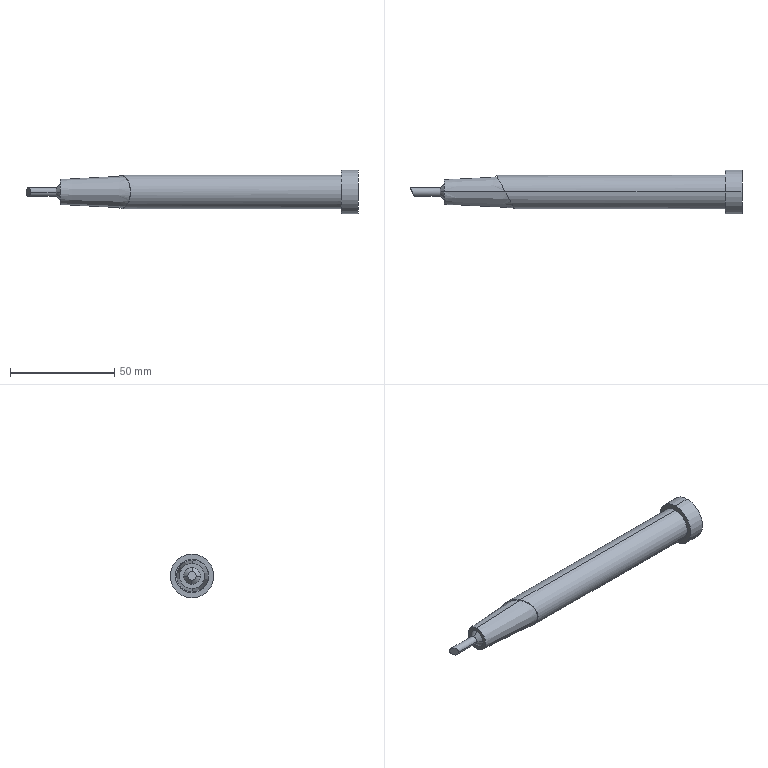Part | Creo | 1 solid | 17 faces | box 159.433 x 21 x 21 mm | volume 28475 mm3 | cylinder 6 | plane 5 | spline 4 | cone 2 | commonest cylinder face diameters 4.02 x2 16 x2 21 x2
STEP:
#1=CARTESIAN_POINT('',(0.,0.,0.));
#2=DIRECTION('',(0.,0.,1.));
#3=DIRECTION('',(1.,0.,0.));
#4=AXIS2_PLACEMENT_3D('',#1,#2,#3);
#5=CARTESIAN_POINT('',(286.206,-41.747,-34.219));
#6=VERTEX_POINT('',#5);
#7=CARTESIAN_POINT('',(290.526,-49.747,-42.219));
#8=VERTEX_POINT('',#7);
#9=CARTESIAN_POINT('',(286.206,-41.747,-34.718));
#10=CARTESIAN_POINT('',(286.256,-41.839,-35.701));
#11=CARTESIAN_POINT('',(286.478,-42.251,-37.148));
#12=CARTESIAN_POINT('',(286.853,-42.944,-38.521));
#13=CARTESIAN_POINT('',(287.359,-43.882,-39.731));
#14=CARTESIAN_POINT('',(287.99,-45.05,-40.76));
#15=CARTESIAN_POINT('',(288.754,-46.465,-41.578));
#16=CARTESIAN_POINT('',(289.619,-48.068,-42.1));
#17=CARTESIAN_POINT('',(290.218,-49.176,-42.219));
#18=CARTESIAN_POINT('',(290.526,-49.747,-42.219));
#19=B_SPLINE_CURVE_WITH_KNOTS('',3,(#5,#9,#10,#11,#12,#13,#14,#15,#16,#17,#18),.UNSPECIFIED.,.F.,.F.,(4,1,1,1,1,1,1,1,4),(0.,0.125,0.25,0.375,0.5,0.625,0.75,0.875,1.),.UNSPECIFIED.);
#20=EDGE_CURVE('',#6,#8,#19,.T.);
#21=ORIENTED_EDGE('',*,*,#20,.T.);
#22=CARTESIAN_POINT('',(396.101,-49.747,-42.219));
#23=VERTEX_POINT('',#22);
#24=CARTESIAN_POINT('',(290.526,-49.747,-42.219));
#25=DIRECTION('',(1.,0.000000001,-0.000000955));
#26=VECTOR('',#25,105.575);
#27=LINE('',#24,#26);
#28=EDGE_CURVE('',#8,#23,#27,.T.);
#29=ORIENTED_EDGE('',*,*,#28,.T.);
#30=CARTESIAN_POINT('',(396.101,-49.747,-26.219));
#31=VERTEX_POINT('',#30);
#32=CARTESIAN_POINT('',(396.101,-49.747,-34.219));
#33=DIRECTION('',(1.,0.,0.));
#34=DIRECTION('',(0.,0.,-1.));
#35=AXIS2_PLACEMENT_3D('',#32,#33,#34);
#36=CIRCLE('',#35,8.);
#37=EDGE_CURVE('',#23,#31,#36,.T.);
#38=ORIENTED_EDGE('',*,*,#37,.T.);
#39=CARTESIAN_POINT('',(290.526,-49.747,-26.219));
#40=VERTEX_POINT('',#39);
#41=CARTESIAN_POINT('',(290.526,-49.747,-26.219));
#42=DIRECTION('',(1.,0.00000261,0.000001073));
#43=VECTOR('',#42,105.574);
#44=LINE('',#41,#43);
#45=EDGE_CURVE('',#40,#31,#44,.T.);
#46=ORIENTED_EDGE('',*,*,#45,.F.);
#47=CARTESIAN_POINT('',(286.206,-41.747,-34.219));
#48=CARTESIAN_POINT('',(286.206,-41.747,-33.949));
#49=CARTESIAN_POINT('',(286.221,-41.774,-33.41));
#50=CARTESIAN_POINT('',(286.287,-41.897,-32.605));
#51=CARTESIAN_POINT('',(286.398,-42.103,-31.812));
#52=CARTESIAN_POINT('',(286.554,-42.391,-31.037));
#53=CARTESIAN_POINT('',(286.755,-42.764,-30.285));
#54=CARTESIAN_POINT('',(287.002,-43.22,-29.566));
#55=CARTESIAN_POINT('',(287.293,-43.76,-28.888));
#56=CARTESIAN_POINT('',(287.629,-44.381,-28.263));
#57=CARTESIAN_POINT('',(288.005,-45.079,-27.7));
#58=CARTESIAN_POINT('',(288.426,-45.858,-27.209));
#59=CARTESIAN_POINT('',(288.829,-46.603,-26.849));
#60=CARTESIAN_POINT('',(289.186,-47.266,-26.604));
#61=CARTESIAN_POINT('',(289.512,-47.869,-26.435));
#62=CARTESIAN_POINT('',(289.805,-48.41,-26.325));
#63=CARTESIAN_POINT('',(290.072,-48.905,-26.259));
#64=CARTESIAN_POINT('',(290.304,-49.335,-26.226));
#65=CARTESIAN_POINT('',(290.454,-49.613,-26.219));
#66=CARTESIAN_POINT('',(290.526,-49.747,-26.219));
#67=B_SPLINE_CURVE_WITH_KNOTS('',3,(#47,#48,#49,#50,#51,#52,#53,#54,#55,#56,#57,#58,#59,#60,#61,#62,#63,#64,#65,#66),.UNSPECIFIED.,.F.,.F.,(4,1,1,1,1,1,1,1,1,1,1,1,1,1,1,1,1,4),(0.,0.05882,0.1176,0.1765,0.2353,0.2941,0.3529,0.4118,0.4706,0.5294,0.5882,0.6471,0.7059,0.7647,0.8235,0.8824,0.9412,1.),.UNSPECIFIED.);
#68=EDGE_CURVE('',#6,#40,#67,.T.);
#69=ORIENTED_EDGE('',*,*,#68,.F.);
#70=EDGE_LOOP('',(#21,#29,#38,#46,#69));
#71=FACE_OUTER_BOUND('',#70,.F.);
#72=CARTESIAN_POINT('',(261.212,-49.747,-34.219));
#73=DIRECTION('',(1.,0.,0.));
#74=DIRECTION('',(0.,0.,-1.));
#75=AXIS2_PLACEMENT_3D('',#72,#73,#74);
#76=CYLINDRICAL_SURFACE('',#75,8.);
#77=ADVANCED_FACE('',(#71),#76,.T.);
#78=ORIENTED_EDGE('',*,*,#68,.T.);
#79=CARTESIAN_POINT('',(294.846,-57.747,-34.219));
#80=VERTEX_POINT('',#79);
#81=CARTESIAN_POINT('',(290.526,-49.747,-26.219));
#82=CARTESIAN_POINT('',(290.694,-50.058,-26.219));
#83=CARTESIAN_POINT('',(291.015,-50.651,-26.255));
#84=CARTESIAN_POINT('',(291.45,-51.458,-26.391));
#85=CARTESIAN_POINT('',(291.825,-52.152,-26.579));
#86=CARTESIAN_POINT('',(292.144,-52.743,-26.793));
#87=CARTESIAN_POINT('',(292.446,-53.301,-27.042));
#88=CARTESIAN_POINT('',(292.779,-53.918,-27.378));
#89=CARTESIAN_POINT('',(293.144,-54.594,-27.835));
#90=CARTESIAN_POINT('',(293.504,-55.261,-28.401));
#91=CARTESIAN_POINT('',(293.822,-55.849,-29.023));
#92=CARTESIAN_POINT('',(294.098,-56.361,-29.693));
#93=CARTESIAN_POINT('',(294.331,-56.793,-30.4));
#94=CARTESIAN_POINT('',(294.521,-57.144,-31.138));
#95=CARTESIAN_POINT('',(294.668,-57.416,-31.896));
#96=CARTESIAN_POINT('',(294.772,-57.61,-32.676));
#97=CARTESIAN_POINT('',(294.833,-57.721,-33.442));
#98=CARTESIAN_POINT('',(294.846,-57.747,-33.96));
#99=CARTESIAN_POINT('',(294.846,-57.747,-34.219));
#100=B_SPLINE_CURVE_WITH_KNOTS('',3,(#81,#82,#83,#84,#85,#86,#87,#88,#89,#90,#91,#92,#93,#94,#95,#96,#97,#98,#99),.UNSPECIFIED.,.F.,.F.,(4,1,1,1,1,1,1,1,1,1,1,1,1,1,1,1,4),(0.,0.0625,0.125,0.1875,0.25,0.3125,0.375,0.4375,0.5,0.5625,0.625,0.6875,0.75,0.8125,0.875,0.9375,1.),.UNSPECIFIED.);
#101=EDGE_CURVE('',#40,#80,#100,.T.);
#102=ORIENTED_EDGE('',*,*,#101,.T.);
#103=CARTESIAN_POINT('',(294.846,-57.747,-34.712));
#104=CARTESIAN_POINT('',(294.798,-57.657,-35.689));
#105=CARTESIAN_POINT('',(294.575,-57.243,-37.153));
#106=CARTESIAN_POINT('',(294.192,-56.535,-38.542));
#107=CARTESIAN_POINT('',(293.697,-55.618,-39.725));
#108=CARTESIAN_POINT('',(293.047,-54.415,-40.782));
#109=CARTESIAN_POINT('',(292.296,-53.023,-41.576));
#110=CARTESIAN_POINT('',(291.458,-51.472,-42.089));
#111=CARTESIAN_POINT('',(290.846,-50.339,-42.219));
#112=CARTESIAN_POINT('',(290.526,-49.747,-42.219));
#113=B_SPLINE_CURVE_WITH_KNOTS('',3,(#79,#103,#104,#105,#106,#107,#108,#109,#110,#111,#112),.UNSPECIFIED.,.F.,.F.,(4,1,1,1,1,1,1,1,4),(0.,0.125,0.25,0.375,0.5,0.625,0.75,0.875,1.),.UNSPECIFIED.);
#114=EDGE_CURVE('',#80,#8,#113,.T.);
#115=ORIENTED_EDGE('',*,*,#114,.T.);
#116=ORIENTED_EDGE('',*,*,#20,.F.);
#117=EDGE_LOOP('',(#78,#102,#115,#116));
#118=FACE_OUTER_BOUND('',#117,.F.);
#119=CARTESIAN_POINT('',(294.715,-57.503,-34.219));
#120=VERTEX_POINT('',#119);
#121=CARTESIAN_POINT('',(290.526,-49.747,-41.755));
#122=VERTEX_POINT('',#121);
#123=CARTESIAN_POINT('',(294.715,-57.503,-34.219));
#124=CARTESIAN_POINT('',(294.715,-57.503,-34.909));
#125=CARTESIAN_POINT('',(294.62,-57.327,-36.086));
#126=CARTESIAN_POINT('',(294.232,-56.608,-38.011));
#127=CARTESIAN_POINT('',(293.479,-55.215,-39.84));
#128=CARTESIAN_POINT('',(292.456,-53.32,-41.085));
#129=CARTESIAN_POINT('',(291.444,-51.446,-41.663));
#130=CARTESIAN_POINT('',(290.854,-50.354,-41.772));
#131=CARTESIAN_POINT('',(290.526,-49.747,-41.755));
#132=B_SPLINE_CURVE_WITH_KNOTS('',3,(#123,#124,#125,#126,#127,#128,#129,#130,#131),.UNSPECIFIED.,.F.,.F.,(4,1,1,1,1,1,4),(0.,0.125,0.25,0.5,0.75,0.875,1.),.UNSPECIFIED.);
#133=EDGE_CURVE('',#120,#122,#132,.T.);
#134=ORIENTED_EDGE('',*,*,#133,.F.);
#135=CARTESIAN_POINT('',(290.526,-49.747,-26.683));
#136=VERTEX_POINT('',#135);
#137=CARTESIAN_POINT('',(294.715,-57.503,-33.528));
#138=CARTESIAN_POINT('',(294.62,-57.327,-32.352));
#139=CARTESIAN_POINT('',(294.232,-56.608,-30.427));
#140=CARTESIAN_POINT('',(293.479,-55.215,-28.598));
#141=CARTESIAN_POINT('',(292.456,-53.32,-27.353));
#142=CARTESIAN_POINT('',(291.444,-51.446,-26.775));
#143=CARTESIAN_POINT('',(290.854,-50.354,-26.665));
#144=CARTESIAN_POINT('',(290.526,-49.747,-26.683));
#145=B_SPLINE_CURVE_WITH_KNOTS('',3,(#119,#137,#138,#139,#140,#141,#142,#143,#144),.UNSPECIFIED.,.F.,.F.,(4,1,1,1,1,1,4),(0.,0.125,0.25,0.5,0.75,0.875,1.),.UNSPECIFIED.);
#146=EDGE_CURVE('',#120,#136,#145,.T.);
#147=ORIENTED_EDGE('',*,*,#146,.T.);
#148=CARTESIAN_POINT('',(290.526,-49.747,-41.755));
#149=CARTESIAN_POINT('',(290.479,-49.66,-41.753));
#150=CARTESIAN_POINT('',(290.425,-49.559,-41.748));
#151=CARTESIAN_POINT('',(290.339,-49.399,-41.738));
#152=CARTESIAN_POINT('',(290.261,-49.256,-41.726));
#153=CARTESIAN_POINT('',(290.185,-49.114,-41.711));
#154=CARTESIAN_POINT('',(290.098,-48.953,-41.691));
#155=CARTESIAN_POINT('',(290.007,-48.785,-41.667));
#156=CARTESIAN_POINT('',(289.914,-48.612,-41.637));
#157=CARTESIAN_POINT('',(289.831,-48.46,-41.608));
#158=CARTESIAN_POINT('',(289.732,-48.276,-41.569));
#159=CARTESIAN_POINT('',(289.623,-48.073,-41.52));
#160=CARTESIAN_POINT('',(289.507,-47.859,-41.461));
#161=CARTESIAN_POINT('',(289.368,-47.602,-41.382));
#162=CARTESIAN_POINT('',(289.216,-47.321,-41.284));
#163=CARTESIAN_POINT('',(289.057,-47.026,-41.166));
#164=CARTESIAN_POINT('',(288.914,-46.762,-41.049));
#165=CARTESIAN_POINT('',(288.785,-46.522,-40.931));
#166=CARTESIAN_POINT('',(288.626,-46.228,-40.774));
#167=CARTESIAN_POINT('',(288.449,-45.9,-40.578));
#168=CARTESIAN_POINT('',(288.262,-45.554,-40.342));
#169=CARTESIAN_POINT('',(288.095,-45.244,-40.107));
#170=CARTESIAN_POINT('',(287.944,-44.965,-39.871));
#171=CARTESIAN_POINT('',(287.807,-44.71,-39.636));
#172=CARTESIAN_POINT('',(287.639,-44.4,-39.322));
#173=CARTESIAN_POINT('',(287.456,-44.061,-38.929));
#174=CARTESIAN_POINT('',(287.269,-43.714,-38.458));
#175=CARTESIAN_POINT('',(287.11,-43.42,-37.987));
#176=CARTESIAN_POINT('',(286.975,-43.171,-37.516));
#177=CARTESIAN_POINT('',(286.825,-42.892,-36.888));
#178=CARTESIAN_POINT('',(286.686,-42.636,-36.103));
#179=CARTESIAN_POINT('',(286.59,-42.457,-35.161));
#180=CARTESIAN_POINT('',(286.558,-42.398,-34.219));
#181=CARTESIAN_POINT('',(286.59,-42.457,-33.277));
#182=CARTESIAN_POINT('',(286.686,-42.636,-32.335));
#183=CARTESIAN_POINT('',(286.825,-42.892,-31.55));
#184=CARTESIAN_POINT('',(286.975,-43.171,-30.922));
#185=CARTESIAN_POINT('',(287.11,-43.42,-30.451));
#186=CARTESIAN_POINT('',(287.269,-43.714,-29.98));
#187=CARTESIAN_POINT('',(287.456,-44.061,-29.509));
#188=CARTESIAN_POINT('',(287.639,-44.4,-29.116));
#189=CARTESIAN_POINT('',(287.807,-44.71,-28.802));
#190=CARTESIAN_POINT('',(287.944,-44.965,-28.567));
#191=CARTESIAN_POINT('',(288.095,-45.244,-28.331));
#192=CARTESIAN_POINT('',(288.262,-45.554,-28.096));
#193=CARTESIAN_POINT('',(288.449,-45.9,-27.86));
#194=CARTESIAN_POINT('',(288.626,-46.228,-27.664));
#195=CARTESIAN_POINT('',(288.785,-46.522,-27.507));
#196=CARTESIAN_POINT('',(288.914,-46.762,-27.389));
#197=CARTESIAN_POINT('',(289.057,-47.026,-27.271));
#198=CARTESIAN_POINT('',(289.216,-47.321,-27.154));
#199=CARTESIAN_POINT('',(289.368,-47.602,-27.056));
#200=CARTESIAN_POINT('',(289.507,-47.859,-26.977));
#201=CARTESIAN_POINT('',(289.623,-48.073,-26.918));
#202=CARTESIAN_POINT('',(289.732,-48.276,-26.869));
#203=CARTESIAN_POINT('',(289.831,-48.46,-26.83));
#204=CARTESIAN_POINT('',(289.914,-48.612,-26.8));
#205=CARTESIAN_POINT('',(290.007,-48.785,-26.771));
#206=CARTESIAN_POINT('',(290.098,-48.953,-26.746));
#207=CARTESIAN_POINT('',(290.185,-49.114,-26.727));
#208=CARTESIAN_POINT('',(290.261,-49.256,-26.712));
#209=CARTESIAN_POINT('',(290.339,-49.399,-26.7));
#210=CARTESIAN_POINT('',(290.425,-49.559,-26.69));
#211=CARTESIAN_POINT('',(290.479,-49.66,-26.685));
#212=CARTESIAN_POINT('',(290.526,-49.747,-26.683));
#213=B_SPLINE_CURVE_WITH_KNOTS('',3,(#148,#149,#150,#151,#152,#153,#154,#155,#156,#157,#158,#159,#160,#161,#162,#163,#164,#165,#166,#167,#168,#169,#170,#171,#172,#173,#174,#175,#176,#177,#178,#179,#180,#181,#182,#183,#184,#185,#186,#187,#188,#189,#190,#191,#192,#193,#194,#195,#196,#197,#198,#199,#200,#201,#202,#203,#204,#205,#206,#207,#208,#209,#210,#211,#212),.UNSPECIFIED.,.F.,.F.,(4,1,1,1,1,1,1,1,1,1,1,1,1,1,1,1,1,1,1,1,1,1,1,1,1,1,1,1,1,1,1,1,1,1,1,1,1,1,1,1,1,1,1,1,1,1,1,1,1,1,1,1,1,1,1,1,1,1,1,1,1,1,4),(0.,0.0004883,0.0009766,0.001953,0.00293,0.003906,0.005859,0.007812,0.009766,0.01172,0.01562,0.01953,0.02344,0.03125,0.03906,0.04688,0.05469,0.0625,0.07812,0.09375,0.1094,0.125,0.1406,0.1562,0.1875,0.2188,0.25,0.2812,0.3125,0.375,0.4375,0.5,0.5625,0.625,0.6875,0.7188,0.75,0.7812,0.8125,0.8438,0.8594,0.875,0.8906,0.9062,0.9219,0.9375,0.9453,0.9531,0.9609,0.9688,0.9766,0.9805,0.9844,0.9883,0.9902,0.9922,0.9941,0.9961,0.9971,0.998,0.999,0.9995,1.),.UNSPECIFIED.);
#214=EDGE_CURVE('',#122,#136,#213,.T.);
#215=ORIENTED_EDGE('',*,*,#214,.F.);
#216=EDGE_LOOP('',(#134,#147,#215));
#217=FACE_BOUND('',#216,.F.);
#218=CARTESIAN_POINT('',(241.82,40.446,-130.777));
#219=DIRECTION('',(-0.8799,-0.4752,-0.000000028));
#220=DIRECTION('',(0.4752,-0.8799,0.));
#221=AXIS2_PLACEMENT_3D('',#218,#219,#220);
#222=PLANE('',#221);
#223=ADVANCED_FACE('',(#118,#217),#222,.T.);
#224=ORIENTED_EDGE('',*,*,#146,.F.);
#225=ORIENTED_EDGE('',*,*,#133,.T.);
#226=CARTESIAN_POINT('',(261.212,-49.747,-40.219));
#227=VERTEX_POINT('',#226);
#228=CARTESIAN_POINT('',(261.212,-49.747,-40.219));
#229=DIRECTION('',(0.9986,0.,-0.05234));
#230=VECTOR('',#229,29.354);
#231=LINE('',#228,#230);
#232=EDGE_CURVE('',#227,#122,#231,.T.);
#233=ORIENTED_EDGE('',*,*,#232,.F.);
#234=CARTESIAN_POINT('',(261.212,-49.747,-28.219));
#235=VERTEX_POINT('',#234);
#236=CARTESIAN_POINT('',(261.212,-49.747,-34.219));
#237=DIRECTION('',(-1.,0.,0.));
#238=DIRECTION('',(0.,0.,-1.));
#239=AXIS2_PLACEMENT_3D('',#236,#237,#238);
#240=CIRCLE('',#239,6.);
#241=EDGE_CURVE('',#227,#235,#240,.T.);
#242=ORIENTED_EDGE('',*,*,#241,.T.);
#243=CARTESIAN_POINT('',(261.212,-49.747,-28.219));
#244=DIRECTION('',(0.9986,0.,0.05234));
#245=VECTOR('',#244,29.354);
#246=LINE('',#243,#245);
#247=EDGE_CURVE('',#235,#136,#246,.T.);
#248=ORIENTED_EDGE('',*,*,#247,.T.);
#249=EDGE_LOOP('',(#224,#225,#233,#242,#248));
#250=FACE_OUTER_BOUND('',#249,.F.);
#251=CARTESIAN_POINT('',(277.963,-49.747,-34.219));
#252=DIRECTION('',(1.,0.,0.));
#253=DIRECTION('',(0.,0.,-1.));
#254=AXIS2_PLACEMENT_3D('',#251,#252,#253);
#255=CONICAL_SURFACE('',#254,6.878,3.);
#256=ADVANCED_FACE('',(#250),#255,.T.);
#257=ORIENTED_EDGE('',*,*,#214,.T.);
#258=ORIENTED_EDGE('',*,*,#247,.F.);
#259=CARTESIAN_POINT('',(261.212,-49.747,-34.219));
#260=DIRECTION('',(-1.,0.,0.));
#261=DIRECTION('',(0.,0.,1.));
#262=AXIS2_PLACEMENT_3D('',#259,#260,#261);
#263=CIRCLE('',#262,6.);
#264=EDGE_CURVE('',#235,#227,#263,.T.);
#265=ORIENTED_EDGE('',*,*,#264,.T.);
#266=ORIENTED_EDGE('',*,*,#232,.T.);
#267=EDGE_LOOP('',(#257,#258,#265,#266));
#268=FACE_OUTER_BOUND('',#267,.F.);
#269=CARTESIAN_POINT('',(275.869,-49.747,-34.219));
#270=DIRECTION('',(1.,0.,0.));
#271=DIRECTION('',(0.,0.,-1.));
#272=AXIS2_PLACEMENT_3D('',#269,#270,#271);
#273=CONICAL_SURFACE('',#272,6.768,3.);
#274=ADVANCED_FACE('',(#268),#273,.T.);
#275=ORIENTED_EDGE('',*,*,#241,.F.);
#276=ORIENTED_EDGE('',*,*,#264,.F.);
#277=EDGE_LOOP('',(#275,#276));
#278=FACE_OUTER_BOUND('',#277,.F.);
#279=CARTESIAN_POINT('',(261.212,-49.747,-30.199));
#280=VERTEX_POINT('',#279);
#281=CARTESIAN_POINT('',(261.212,-53.767,-34.219));
#282=VERTEX_POINT('',#281);
#283=CARTESIAN_POINT('',(261.212,-50.104,-30.199));
#284=CARTESIAN_POINT('',(261.212,-50.793,-30.295));
#285=CARTESIAN_POINT('',(261.212,-51.777,-30.702));
#286=CARTESIAN_POINT('',(261.212,-52.629,-31.351));
#287=CARTESIAN_POINT('',(261.212,-53.273,-32.203));
#288=CARTESIAN_POINT('',(261.212,-53.673,-33.183));
#289=CARTESIAN_POINT('',(261.212,-53.767,-33.866));
#290=CARTESIAN_POINT('',(261.212,-53.767,-34.219));
#291=B_SPLINE_CURVE_WITH_KNOTS('',3,(#279,#283,#284,#285,#286,#287,#288,#289,#290),.UNSPECIFIED.,.F.,.F.,(4,1,1,1,1,1,4),(0.,0.1667,0.3333,0.5,0.6667,0.8333,1.),.UNSPECIFIED.);
#292=EDGE_CURVE('',#280,#282,#291,.T.);
#293=ORIENTED_EDGE('',*,*,#292,.F.);
#294=CARTESIAN_POINT('',(261.212,-48.134,-30.537));
#295=VERTEX_POINT('',#294);
#296=CARTESIAN_POINT('',(261.212,-48.628,-30.32));
#297=CARTESIAN_POINT('',(261.212,-49.174,-30.199));
#298=CARTESIAN_POINT('',(261.212,-49.747,-30.199));
#299=B_SPLINE_CURVE_WITH_KNOTS('',3,(#294,#296,#297,#298),.UNSPECIFIED.,.F.,.F.,(4,4),(0.,1.),.UNSPECIFIED.);
#300=EDGE_CURVE('',#295,#280,#299,.T.);
#301=ORIENTED_EDGE('',*,*,#300,.F.);
#302=CARTESIAN_POINT('',(261.212,-46.588,-31.737));
#303=VERTEX_POINT('',#302);
#304=CARTESIAN_POINT('',(261.212,-46.994,-31.22));
#305=CARTESIAN_POINT('',(261.212,-47.525,-30.805));
#306=CARTESIAN_POINT('',(261.212,-48.134,-30.537));
#307=B_SPLINE_CURVE_WITH_KNOTS('',3,(#302,#304,#305,#306),.UNSPECIFIED.,.F.,.F.,(4,4),(0.,1.),.UNSPECIFIED.);
#308=EDGE_CURVE('',#303,#295,#307,.T.);
#309=ORIENTED_EDGE('',*,*,#308,.F.);
#310=CARTESIAN_POINT('',(261.212,-45.727,-34.219));
#311=VERTEX_POINT('',#310);
#312=CARTESIAN_POINT('',(261.212,-45.727,-33.917));
#313=CARTESIAN_POINT('',(261.212,-45.793,-33.33));
#314=CARTESIAN_POINT('',(261.212,-46.089,-32.476));
#315=CARTESIAN_POINT('',(261.212,-46.401,-31.974));
#316=CARTESIAN_POINT('',(261.212,-46.588,-31.737));
#317=B_SPLINE_CURVE_WITH_KNOTS('',3,(#310,#312,#313,#314,#315,#316),.UNSPECIFIED.,.F.,.F.,(4,1,1,4),(0.,0.3333,0.6667,1.),.UNSPECIFIED.);
#318=EDGE_CURVE('',#311,#303,#317,.T.);
#319=ORIENTED_EDGE('',*,*,#318,.F.);
#320=CARTESIAN_POINT('',(261.212,-49.747,-38.239));
#321=VERTEX_POINT('',#320);
#322=CARTESIAN_POINT('',(261.212,-49.39,-38.239));
#323=CARTESIAN_POINT('',(261.212,-48.701,-38.143));
#324=CARTESIAN_POINT('',(261.212,-47.717,-37.736));
#325=CARTESIAN_POINT('',(261.212,-46.864,-37.086));
#326=CARTESIAN_POINT('',(261.212,-46.221,-36.235));
#327=CARTESIAN_POINT('',(261.212,-45.82,-35.255));
#328=CARTESIAN_POINT('',(261.212,-45.727,-34.572));
#329=CARTESIAN_POINT('',(261.212,-45.727,-34.219));
#330=B_SPLINE_CURVE_WITH_KNOTS('',3,(#320,#322,#323,#324,#325,#326,#327,#328,#329),.UNSPECIFIED.,.F.,.F.,(4,1,1,1,1,1,4),(0.,0.1667,0.3333,0.5,0.6667,0.8333,1.),.UNSPECIFIED.);
#331=EDGE_CURVE('',#321,#311,#330,.T.);
#332=ORIENTED_EDGE('',*,*,#331,.F.);
#333=CARTESIAN_POINT('',(261.212,-53.767,-34.219));
#334=CARTESIAN_POINT('',(261.212,-53.767,-34.576));
#335=CARTESIAN_POINT('',(261.212,-53.671,-35.265));
#336=CARTESIAN_POINT('',(261.212,-53.264,-36.249));
#337=CARTESIAN_POINT('',(261.212,-52.614,-37.101));
#338=CARTESIAN_POINT('',(261.212,-51.763,-37.745));
#339=CARTESIAN_POINT('',(261.212,-50.783,-38.145));
#340=CARTESIAN_POINT('',(261.212,-50.1,-38.239));
#341=CARTESIAN_POINT('',(261.212,-49.747,-38.239));
#342=B_SPLINE_CURVE_WITH_KNOTS('',3,(#333,#334,#335,#336,#337,#338,#339,#340,#341),.UNSPECIFIED.,.F.,.F.,(4,1,1,1,1,1,4),(0.,0.1667,0.3333,0.5,0.6667,0.8333,1.),.UNSPECIFIED.);
#343=EDGE_CURVE('',#282,#321,#342,.T.);
#344=ORIENTED_EDGE('',*,*,#343,.F.);
#345=EDGE_LOOP('',(#293,#301,#309,#319,#332,#344));
#346=FACE_BOUND('',#345,.F.);
#347=CARTESIAN_POINT('',(261.212,-27.098,-27.127));
#348=DIRECTION('',(1.,-0.000000001,-0.00000112));
#349=DIRECTION('',(-0.00000112,0.,-1.));
#350=AXIS2_PLACEMENT_3D('',#347,#348,#349);
#351=PLANE('',#350);
#352=ADVANCED_FACE('',(#278,#346),#351,.F.);
#353=CARTESIAN_POINT('',(259.202,-49.747,-32.209));
#354=VERTEX_POINT('',#353);
#355=CARTESIAN_POINT('',(259.202,-51.757,-34.219));
#356=VERTEX_POINT('',#355);
#357=CARTESIAN_POINT('',(259.202,-49.747,-32.209));
#358=CARTESIAN_POINT('',(259.202,-49.959,-32.209));
#359=CARTESIAN_POINT('',(259.202,-50.381,-32.277));
#360=CARTESIAN_POINT('',(259.203,-50.949,-32.567));
#361=CARTESIAN_POINT('',(259.203,-51.399,-33.017));
#362=CARTESIAN_POINT('',(259.202,-51.689,-33.584));
#363=CARTESIAN_POINT('',(259.202,-51.757,-34.007));
#364=CARTESIAN_POINT('',(259.202,-51.757,-34.219));
#365=B_SPLINE_CURVE_WITH_KNOTS('',3,(#357,#358,#359,#360,#361,#362,#363,#364),.UNSPECIFIED.,.F.,.F.,(4,1,1,1,1,4),(0.,0.2,0.4,0.6,0.8,1.),.UNSPECIFIED.);
#366=EDGE_CURVE('',#354,#356,#365,.T.);
#367=ORIENTED_EDGE('',*,*,#366,.F.);
#368=CARTESIAN_POINT('',(261.212,-49.747,-30.199));
#369=DIRECTION('',(-0.7071,0.000000043,-0.7071));
#370=VECTOR('',#369,2.843);
#371=LINE('',#368,#370);
#372=EDGE_CURVE('',#280,#354,#371,.T.);
#373=ORIENTED_EDGE('',*,*,#372,.F.);
#374=ORIENTED_EDGE('',*,*,#292,.T.);
#375=CARTESIAN_POINT('',(259.202,-51.757,-34.219));
#376=DIRECTION('',(0.7071,-0.7071,-0.0000061));
#377=VECTOR('',#376,2.843);
#378=LINE('',#375,#377);
#379=EDGE_CURVE('',#356,#282,#378,.T.);
#380=ORIENTED_EDGE('',*,*,#379,.F.);
#381=EDGE_LOOP('',(#367,#373,#374,#380));
#382=FACE_OUTER_BOUND('',#381,.F.);
#383=CARTESIAN_POINT('',(259.064,-51.617,-34.305));
#384=CARTESIAN_POINT('',(259.826,-52.378,-34.34));
#385=CARTESIAN_POINT('',(260.588,-53.139,-34.375));
#386=CARTESIAN_POINT('',(261.35,-53.9,-34.41));
#387=CARTESIAN_POINT('',(259.064,-51.618,-34.276));
#388=CARTESIAN_POINT('',(259.826,-52.38,-34.3));
#389=CARTESIAN_POINT('',(260.588,-53.141,-34.323));
#390=CARTESIAN_POINT('',(261.35,-53.903,-34.346));
#391=CARTESIAN_POINT('',(259.064,-51.642,-33.21));
#392=CARTESIAN_POINT('',(259.826,-52.413,-32.8));
#393=CARTESIAN_POINT('',(260.588,-53.185,-32.389));
#394=CARTESIAN_POINT('',(261.35,-53.956,-31.979));
#395=CARTESIAN_POINT('',(259.064,-50.755,-32.323));
#396=CARTESIAN_POINT('',(259.826,-51.165,-31.552));
#397=CARTESIAN_POINT('',(260.588,-51.575,-30.78));
#398=CARTESIAN_POINT('',(261.35,-51.986,-30.009));
#399=CARTESIAN_POINT('',(259.064,-49.689,-32.347));
#400=CARTESIAN_POINT('',(259.826,-49.665,-31.586));
#401=CARTESIAN_POINT('',(260.588,-49.642,-30.824));
#402=CARTESIAN_POINT('',(261.35,-49.618,-30.063));
#403=CARTESIAN_POINT('',(259.064,-49.66,-32.349));
#404=CARTESIAN_POINT('',(259.826,-49.624,-31.588));
#405=CARTESIAN_POINT('',(260.588,-49.589,-30.827));
#406=CARTESIAN_POINT('',(261.35,-49.554,-30.066));
#407=B_SPLINE_SURFACE_WITH_KNOTS('',3,3,((#383,#384,#385,#386),(#387,#388,#389,#390),(#391,#392,#393,#394),(#395,#396,#397,#398),(#399,#400,#401,#402),(#403,#404,#405,#406)),.UNSPECIFIED.,.F.,.F.,.F.,(4,1,1,4),(4,4),(-0.02768,0.,1.,1.028),(-0.06858,1.068),.UNSPECIFIED.);
#408=ADVANCED_FACE('',(#382),#407,.F.);
#409=ORIENTED_EDGE('',*,*,#366,.T.);
#410=CARTESIAN_POINT('',(246.838,-51.757,-34.219));
#411=VERTEX_POINT('',#410);
#412=CARTESIAN_POINT('',(246.838,-51.757,-34.219));
#413=DIRECTION('',(1.,-0.000000968,-0.00000002));
#414=VECTOR('',#413,12.364);
#415=LINE('',#412,#414);
#416=EDGE_CURVE('',#411,#356,#415,.T.);
#417=ORIENTED_EDGE('',*,*,#416,.F.);
#418=CARTESIAN_POINT('',(246.647,-51.403,-33.08));
#419=VERTEX_POINT('',#418);
#420=CARTESIAN_POINT('',(246.838,-51.757,-34.219));
#421=CARTESIAN_POINT('',(246.838,-51.757,-34.085));
#422=CARTESIAN_POINT('',(246.825,-51.731,-33.821));
#423=CARTESIAN_POINT('',(246.76,-51.612,-33.439));
#424=CARTESIAN_POINT('',(246.69,-51.483,-33.196));
#425=B_SPLINE_CURVE_WITH_KNOTS('',3,(#420,#421,#422,#423,#424,#418),.UNSPECIFIED.,.F.,.F.,(4,1,1,4),(0.,0.3333,0.6667,1.),.UNSPECIFIED.);
#426=EDGE_CURVE('',#411,#419,#425,.T.);
#427=ORIENTED_EDGE('',*,*,#426,.T.);
#428=CARTESIAN_POINT('',(246.507,-51.143,-32.773));
#429=VERTEX_POINT('',#428);
#430=CARTESIAN_POINT('',(246.647,-51.403,-33.08));
#431=CARTESIAN_POINT('',(246.605,-51.325,-32.967));
#432=CARTESIAN_POINT('',(246.559,-51.239,-32.865));
#433=B_SPLINE_CURVE_WITH_KNOTS('',3,(#430,#431,#432,#428),.UNSPECIFIED.,.F.,.F.,(4,4),(0.,1.),.UNSPECIFIED.);
#434=EDGE_CURVE('',#419,#429,#433,.T.);
#435=ORIENTED_EDGE('',*,*,#434,.T.);
#436=CARTESIAN_POINT('',(244.667,-47.737,-34.219));
#437=VERTEX_POINT('',#436);
#438=CARTESIAN_POINT('',(246.507,-51.143,-32.773));
#439=CARTESIAN_POINT('',(246.429,-50.998,-32.633));
#440=CARTESIAN_POINT('',(246.257,-50.68,-32.406));
#441=CARTESIAN_POINT('',(245.944,-50.101,-32.209));
#442=CARTESIAN_POINT('',(245.61,-49.482,-32.195));
#443=CARTESIAN_POINT('',(245.286,-48.882,-32.371));
#444=CARTESIAN_POINT('',(245.013,-48.376,-32.71));
#445=CARTESIAN_POINT('',(244.812,-48.004,-33.166));
#446=CARTESIAN_POINT('',(244.693,-47.784,-33.684));
#447=CARTESIAN_POINT('',(244.667,-47.737,-34.037));
#448=CARTESIAN_POINT('',(244.667,-47.737,-34.219));
#449=B_SPLINE_CURVE_WITH_KNOTS('',3,(#438,#439,#440,#441,#442,#443,#444,#445,#446,#447,#448),.UNSPECIFIED.,.F.,.F.,(4,1,1,1,1,1,1,1,4),(0.,0.125,0.25,0.375,0.5,0.625,0.75,0.875,1.),.UNSPECIFIED.);
#450=EDGE_CURVE('',#429,#437,#449,.T.);
#451=ORIENTED_EDGE('',*,*,#450,.T.);
#452=CARTESIAN_POINT('',(259.202,-47.737,-34.219));
#453=VERTEX_POINT('',#452);
#454=CARTESIAN_POINT('',(244.667,-47.737,-34.219));
#455=DIRECTION('',(1.,-0.000001399,0.000000006));
#456=VECTOR('',#455,14.534);
#457=LINE('',#454,#456);
#458=EDGE_CURVE('',#437,#453,#457,.T.);
#459=ORIENTED_EDGE('',*,*,#458,.T.);
#460=CARTESIAN_POINT('',(259.202,-47.737,-34.219));
#461=CARTESIAN_POINT('',(259.202,-47.737,-34.007));
#462=CARTESIAN_POINT('',(259.202,-47.804,-33.584));
#463=CARTESIAN_POINT('',(259.203,-48.095,-33.017));
#464=CARTESIAN_POINT('',(259.203,-48.545,-32.567));
#465=CARTESIAN_POINT('',(259.202,-49.112,-32.277));
#466=CARTESIAN_POINT('',(259.202,-49.535,-32.209));
#467=CARTESIAN_POINT('',(259.202,-49.747,-32.209));
#468=B_SPLINE_CURVE_WITH_KNOTS('',3,(#460,#461,#462,#463,#464,#465,#466,#467),.UNSPECIFIED.,.F.,.F.,(4,1,1,1,1,4),(0.,0.2,0.4,0.6,0.8,1.),.UNSPECIFIED.);
#469=EDGE_CURVE('',#453,#354,#468,.T.);
#470=ORIENTED_EDGE('',*,*,#469,.T.);
#471=EDGE_LOOP('',(#409,#417,#427,#435,#451,#459,#470));
#472=FACE_OUTER_BOUND('',#471,.F.);
#473=CARTESIAN_POINT('',(245.672,-49.747,-34.219));
#474=DIRECTION('',(1.,0.,0.));
#475=DIRECTION('',(0.,1.,0.));
#476=AXIS2_PLACEMENT_3D('',#473,#474,#475);
#477=CYLINDRICAL_SURFACE('',#476,2.01);
#478=ADVANCED_FACE('',(#472),#477,.T.);
#479=CARTESIAN_POINT('',(259.202,-49.747,-36.229));
#480=VERTEX_POINT('',#479);
#481=CARTESIAN_POINT('',(259.202,-49.747,-36.229));
#482=CARTESIAN_POINT('',(259.202,-49.535,-36.229));
#483=CARTESIAN_POINT('',(259.202,-49.112,-36.161));
#484=CARTESIAN_POINT('',(259.203,-48.545,-35.871));
#485=CARTESIAN_POINT('',(259.203,-48.095,-35.421));
#486=CARTESIAN_POINT('',(259.202,-47.804,-34.853));
#487=CARTESIAN_POINT('',(259.202,-47.737,-34.431));
#488=CARTESIAN_POINT('',(259.202,-47.737,-34.219));
#489=B_SPLINE_CURVE_WITH_KNOTS('',3,(#481,#482,#483,#484,#485,#486,#487,#488),.UNSPECIFIED.,.F.,.F.,(4,1,1,1,1,4),(0.,0.2,0.4,0.6,0.8,1.),.UNSPECIFIED.);
#490=EDGE_CURVE('',#480,#453,#489,.T.);
#491=ORIENTED_EDGE('',*,*,#490,.T.);
#492=ORIENTED_EDGE('',*,*,#458,.F.);
#493=CARTESIAN_POINT('',(244.667,-47.737,-34.219));
#494=CARTESIAN_POINT('',(244.667,-47.737,-34.401));
#495=CARTESIAN_POINT('',(244.693,-47.785,-34.752));
#496=CARTESIAN_POINT('',(244.806,-47.993,-35.251));
#497=CARTESIAN_POINT('',(244.991,-48.336,-35.686));
#498=CARTESIAN_POINT('',(245.246,-48.808,-36.028));
#499=CARTESIAN_POINT('',(245.556,-49.381,-36.226));
#500=CARTESIAN_POINT('',(245.891,-50.003,-36.244));
#501=CARTESIAN_POINT('',(246.218,-50.608,-36.071));
#502=CARTESIAN_POINT('',(246.495,-51.122,-35.726));
#503=CARTESIAN_POINT('',(246.693,-51.488,-35.275));
#504=CARTESIAN_POINT('',(246.812,-51.708,-34.759));
#505=CARTESIAN_POINT('',(246.838,-51.757,-34.403));
#506=CARTESIAN_POINT('',(246.838,-51.757,-34.219));
#507=B_SPLINE_CURVE_WITH_KNOTS('',3,(#493,#494,#495,#496,#497,#498,#499,#500,#501,#502,#503,#504,#505,#506),.UNSPECIFIED.,.F.,.F.,(4,1,1,1,1,1,1,1,1,1,1,4),(0.,0.09091,0.1818,0.2727,0.3636,0.4545,0.5455,0.6364,0.7273,0.8182,0.9091,1.),.UNSPECIFIED.);
#508=EDGE_CURVE('',#437,#411,#507,.T.);
#509=ORIENTED_EDGE('',*,*,#508,.T.);
#510=ORIENTED_EDGE('',*,*,#416,.T.);
#511=CARTESIAN_POINT('',(259.202,-51.757,-34.219));
#512=CARTESIAN_POINT('',(259.202,-51.757,-34.431));
#513=CARTESIAN_POINT('',(259.202,-51.689,-34.853));
#514=CARTESIAN_POINT('',(259.203,-51.399,-35.421));
#515=CARTESIAN_POINT('',(259.203,-50.949,-35.871));
#516=CARTESIAN_POINT('',(259.202,-50.381,-36.161));
#517=CARTESIAN_POINT('',(259.202,-49.959,-36.229));
#518=CARTESIAN_POINT('',(259.202,-49.747,-36.229));
#519=B_SPLINE_CURVE_WITH_KNOTS('',3,(#511,#512,#513,#514,#515,#516,#517,#518),.UNSPECIFIED.,.F.,.F.,(4,1,1,1,1,4),(0.,0.2,0.4,0.6,0.8,1.),.UNSPECIFIED.);
#520=EDGE_CURVE('',#356,#480,#519,.T.);
#521=ORIENTED_EDGE('',*,*,#520,.T.);
#522=EDGE_LOOP('',(#491,#492,#509,#510,#521));
#523=FACE_OUTER_BOUND('',#522,.F.);
#524=CARTESIAN_POINT('',(245.672,-49.747,-34.219));
#525=DIRECTION('',(1.,0.,0.));
#526=DIRECTION('',(0.,1.,0.));
#527=AXIS2_PLACEMENT_3D('',#524,#525,#526);
#528=CYLINDRICAL_SURFACE('',#527,2.01);
#529=ADVANCED_FACE('',(#523),#528,.T.);
#530=ORIENTED_EDGE('',*,*,#490,.F.);
#531=CARTESIAN_POINT('',(259.202,-49.747,-36.229));
#532=DIRECTION('',(0.7071,0.00001227,-0.7071));
#533=VECTOR('',#532,2.843);
#534=LINE('',#531,#533);
#535=EDGE_CURVE('',#480,#321,#534,.T.);
#536=ORIENTED_EDGE('',*,*,#535,.T.);
#537=ORIENTED_EDGE('',*,*,#331,.T.);
#538=CARTESIAN_POINT('',(259.202,-47.737,-34.219));
#539=DIRECTION('',(0.7071,0.7071,-0.000001532));
#540=VECTOR('',#539,2.843);
#541=LINE('',#538,#540);
#542=EDGE_CURVE('',#453,#311,#541,.T.);
#543=ORIENTED_EDGE('',*,*,#542,.F.);
#544=EDGE_LOOP('',(#530,#536,#537,#543));
#545=FACE_OUTER_BOUND('',#544,.F.);
#546=CARTESIAN_POINT('',(259.064,-47.877,-34.133));
#547=CARTESIAN_POINT('',(259.826,-47.116,-34.098));
#548=CARTESIAN_POINT('',(260.588,-46.354,-34.063));
#549=CARTESIAN_POINT('',(261.35,-45.593,-34.028));
#550=CARTESIAN_POINT('',(259.064,-47.875,-34.162));
#551=CARTESIAN_POINT('',(259.826,-47.114,-34.138));
#552=CARTESIAN_POINT('',(260.588,-46.352,-34.115));
#553=CARTESIAN_POINT('',(261.35,-45.591,-34.092));
#554=CARTESIAN_POINT('',(259.064,-47.851,-35.228));
#555=CARTESIAN_POINT('',(259.826,-47.08,-35.638));
#556=CARTESIAN_POINT('',(260.588,-46.309,-36.048));
#557=CARTESIAN_POINT('',(261.35,-45.537,-36.459));
#558=CARTESIAN_POINT('',(259.064,-48.739,-36.115));
#559=CARTESIAN_POINT('',(259.826,-48.328,-36.886));
#560=CARTESIAN_POINT('',(260.588,-47.918,-37.657));
#561=CARTESIAN_POINT('',(261.35,-47.508,-38.429));
#562=CARTESIAN_POINT('',(259.064,-49.805,-36.09));
#563=CARTESIAN_POINT('',(259.826,-49.828,-36.852));
#564=CARTESIAN_POINT('',(260.588,-49.852,-37.614));
#565=CARTESIAN_POINT('',(261.35,-49.875,-38.375));
#566=CARTESIAN_POINT('',(259.064,-49.834,-36.089));
#567=CARTESIAN_POINT('',(259.826,-49.869,-36.85));
#568=CARTESIAN_POINT('',(260.588,-49.905,-37.611));
#569=CARTESIAN_POINT('',(261.35,-49.94,-38.372));
#570=B_SPLINE_SURFACE_WITH_KNOTS('',3,3,((#546,#547,#548,#549),(#550,#551,#552,#553),(#554,#555,#556,#557),(#558,#559,#560,#561),(#562,#563,#564,#565),(#566,#567,#568,#569)),.UNSPECIFIED.,.F.,.F.,.F.,(4,1,1,4),(4,4),(-0.02768,0.,1.,1.028),(-0.06858,1.068),.UNSPECIFIED.);
#571=ADVANCED_FACE('',(#545),#570,.F.);
#572=ORIENTED_EDGE('',*,*,#520,.F.);
#573=ORIENTED_EDGE('',*,*,#379,.T.);
#574=ORIENTED_EDGE('',*,*,#343,.T.);
#575=ORIENTED_EDGE('',*,*,#535,.F.);
#576=EDGE_LOOP('',(#572,#573,#574,#575));
#577=FACE_OUTER_BOUND('',#576,.F.);
#578=CARTESIAN_POINT('',(259.064,-49.661,-36.089));
#579=CARTESIAN_POINT('',(259.826,-49.626,-36.85));
#580=CARTESIAN_POINT('',(260.588,-49.591,-37.611));
#581=CARTESIAN_POINT('',(261.35,-49.556,-38.372));
#582=CARTESIAN_POINT('',(259.064,-49.689,-36.09));
#583=CARTESIAN_POINT('',(259.826,-49.666,-36.852));
#584=CARTESIAN_POINT('',(260.588,-49.643,-37.614));
#585=CARTESIAN_POINT('',(261.35,-49.62,-38.375));
#586=CARTESIAN_POINT('',(259.064,-50.755,-36.114));
#587=CARTESIAN_POINT('',(259.826,-51.166,-36.886));
#588=CARTESIAN_POINT('',(260.588,-51.576,-37.657));
#589=CARTESIAN_POINT('',(261.35,-51.987,-38.428));
#590=CARTESIAN_POINT('',(259.064,-51.642,-35.227));
#591=CARTESIAN_POINT('',(259.826,-52.414,-35.637));
#592=CARTESIAN_POINT('',(260.588,-53.185,-36.048));
#593=CARTESIAN_POINT('',(261.35,-53.957,-36.458));
#594=CARTESIAN_POINT('',(259.064,-51.618,-34.161));
#595=CARTESIAN_POINT('',(259.826,-52.38,-34.138));
#596=CARTESIAN_POINT('',(260.588,-53.141,-34.114));
#597=CARTESIAN_POINT('',(261.35,-53.903,-34.09));
#598=CARTESIAN_POINT('',(259.064,-51.617,-34.132));
#599=CARTESIAN_POINT('',(259.826,-52.378,-34.097));
#600=CARTESIAN_POINT('',(260.588,-53.139,-34.061));
#601=CARTESIAN_POINT('',(261.35,-53.9,-34.026));
#602=B_SPLINE_SURFACE_WITH_KNOTS('',3,3,((#578,#579,#580,#581),(#582,#583,#584,#585),(#586,#587,#588,#589),(#590,#591,#592,#593),(#594,#595,#596,#597),(#598,#599,#600,#601)),.UNSPECIFIED.,.F.,.F.,.F.,(4,1,1,4),(4,4),(-0.02768,0.,1.,1.028),(-0.06858,1.068),.UNSPECIFIED.);
#603=ADVANCED_FACE('',(#577),#602,.F.);
#604=ORIENTED_EDGE('',*,*,#469,.F.);
#605=ORIENTED_EDGE('',*,*,#542,.T.);
#606=ORIENTED_EDGE('',*,*,#318,.T.);
#607=ORIENTED_EDGE('',*,*,#308,.T.);
#608=ORIENTED_EDGE('',*,*,#300,.T.);
#609=ORIENTED_EDGE('',*,*,#372,.T.);
#610=EDGE_LOOP('',(#604,#605,#606,#607,#608,#609));
#611=FACE_OUTER_BOUND('',#610,.F.);
#612=CARTESIAN_POINT('',(259.064,-49.833,-32.349));
#613=CARTESIAN_POINT('',(259.826,-49.868,-31.588));
#614=CARTESIAN_POINT('',(260.588,-49.903,-30.827));
#615=CARTESIAN_POINT('',(261.35,-49.938,-30.065));
#616=CARTESIAN_POINT('',(259.064,-49.804,-32.347));
#617=CARTESIAN_POINT('',(259.826,-49.827,-31.586));
#618=CARTESIAN_POINT('',(260.588,-49.851,-30.824));
#619=CARTESIAN_POINT('',(261.35,-49.874,-30.063));
#620=CARTESIAN_POINT('',(259.064,-48.738,-32.324));
#621=CARTESIAN_POINT('',(259.826,-48.328,-31.552));
#622=CARTESIAN_POINT('',(260.588,-47.917,-30.781));
#623=CARTESIAN_POINT('',(261.35,-47.507,-30.01));
#624=CARTESIAN_POINT('',(259.064,-47.851,-33.211));
#625=CARTESIAN_POINT('',(259.826,-47.08,-32.801));
#626=CARTESIAN_POINT('',(260.588,-46.308,-32.39));
#627=CARTESIAN_POINT('',(261.35,-45.537,-31.98));
#628=CARTESIAN_POINT('',(259.064,-47.875,-34.277));
#629=CARTESIAN_POINT('',(259.826,-47.114,-34.3));
#630=CARTESIAN_POINT('',(260.588,-46.352,-34.324));
#631=CARTESIAN_POINT('',(261.35,-45.59,-34.347));
#632=CARTESIAN_POINT('',(259.064,-47.877,-34.306));
#633=CARTESIAN_POINT('',(259.826,-47.116,-34.341));
#634=CARTESIAN_POINT('',(260.588,-46.354,-34.377));
#635=CARTESIAN_POINT('',(261.35,-45.593,-34.412));
#636=B_SPLINE_SURFACE_WITH_KNOTS('',3,3,((#612,#613,#614,#615),(#616,#617,#618,#619),(#620,#621,#622,#623),(#624,#625,#626,#627),(#628,#629,#630,#631),(#632,#633,#634,#635)),.UNSPECIFIED.,.F.,.F.,.F.,(4,1,1,4),(4,4),(-0.02768,0.,1.,1.028),(-0.06858,1.069),.UNSPECIFIED.);
#637=ADVANCED_FACE('',(#611),#636,.F.);
#638=ORIENTED_EDGE('',*,*,#426,.F.);
#639=ORIENTED_EDGE('',*,*,#508,.F.);
#640=ORIENTED_EDGE('',*,*,#450,.F.);
#641=ORIENTED_EDGE('',*,*,#434,.F.);
#642=EDGE_LOOP('',(#638,#639,#640,#641));
#643=FACE_OUTER_BOUND('',#642,.F.);
#644=CARTESIAN_POINT('',(239.719,-38.574,-41.231));
#645=DIRECTION('',(-0.8799,-0.4752,-0.000000028));
#646=DIRECTION('',(0.4752,-0.8799,0.));
#647=AXIS2_PLACEMENT_3D('',#644,#645,#646);
#648=PLANE('',#647);
#649=ADVANCED_FACE('',(#643),#648,.T.);
#650=ORIENTED_EDGE('',*,*,#114,.F.);
#651=ORIENTED_EDGE('',*,*,#101,.F.);
#652=ORIENTED_EDGE('',*,*,#45,.T.);
#653=CARTESIAN_POINT('',(396.101,-49.747,-34.219));
#654=DIRECTION('',(1.,0.,0.));
#655=DIRECTION('',(0.,0.,1.));
#656=AXIS2_PLACEMENT_3D('',#653,#654,#655);
#657=CIRCLE('',#656,8.);
#658=EDGE_CURVE('',#31,#23,#657,.T.);
#659=ORIENTED_EDGE('',*,*,#658,.T.);
#660=ORIENTED_EDGE('',*,*,#28,.F.);
#661=EDGE_LOOP('',(#650,#651,#652,#659,#660));
#662=FACE_OUTER_BOUND('',#661,.F.);
#663=CARTESIAN_POINT('',(261.212,-49.747,-34.219));
#664=DIRECTION('',(1.,0.,0.));
#665=DIRECTION('',(0.,0.,-1.));
#666=AXIS2_PLACEMENT_3D('',#663,#664,#665);
#667=CYLINDRICAL_SURFACE('',#666,8.);
#668=ADVANCED_FACE('',(#662),#667,.T.);
#669=CARTESIAN_POINT('',(396.101,-49.747,-44.719));
#670=VERTEX_POINT('',#669);
#671=CARTESIAN_POINT('',(396.101,-49.747,-23.719));
#672=VERTEX_POINT('',#671);
#673=CARTESIAN_POINT('',(396.101,-49.747,-34.219));
#674=DIRECTION('',(-1.,0.,0.));
#675=DIRECTION('',(0.,0.,-1.));
#676=AXIS2_PLACEMENT_3D('',#673,#674,#675);
#677=CIRCLE('',#676,10.5);
#678=EDGE_CURVE('',#670,#672,#677,.T.);
#679=ORIENTED_EDGE('',*,*,#678,.F.);
#680=CARTESIAN_POINT('',(396.101,-49.747,-34.219));
#681=DIRECTION('',(-1.,0.,0.));
#682=DIRECTION('',(0.,0.,1.));
#683=AXIS2_PLACEMENT_3D('',#680,#681,#682);
#684=CIRCLE('',#683,10.5);
#685=EDGE_CURVE('',#672,#670,#684,.T.);
#686=ORIENTED_EDGE('',*,*,#685,.F.);
#687=EDGE_LOOP('',(#679,#686));
#688=FACE_OUTER_BOUND('',#687,.F.);
#689=ORIENTED_EDGE('',*,*,#37,.F.);
#690=ORIENTED_EDGE('',*,*,#658,.F.);
#691=EDGE_LOOP('',(#689,#690));
#692=FACE_BOUND('',#691,.F.);
#693=CARTESIAN_POINT('',(396.101,-49.747,-34.219));
#694=DIRECTION('',(1.,0.,0.));
#695=DIRECTION('',(0.,0.,-1.));
#696=AXIS2_PLACEMENT_3D('',#693,#694,#695);
#697=PLANE('',#696);
#698=ADVANCED_FACE('',(#688,#692),#697,.F.);
#699=ORIENTED_EDGE('',*,*,#678,.T.);
#700=CARTESIAN_POINT('',(404.101,-49.747,-23.719));
#701=VERTEX_POINT('',#700);
#702=CARTESIAN_POINT('',(396.101,-49.747,-23.719));
#703=DIRECTION('',(1.,0.,0.));
#704=VECTOR('',#703,8.);
#705=LINE('',#702,#704);
#706=EDGE_CURVE('',#672,#701,#705,.T.);
#707=ORIENTED_EDGE('',*,*,#706,.T.);
#708=CARTESIAN_POINT('',(404.101,-49.747,-44.719));
#709=VERTEX_POINT('',#708);
#710=CARTESIAN_POINT('',(404.101,-49.747,-34.219));
#711=DIRECTION('',(1.,0.,0.));
#712=DIRECTION('',(0.,0.,1.));
#713=AXIS2_PLACEMENT_3D('',#710,#711,#712);
#714=CIRCLE('',#713,10.5);
#715=EDGE_CURVE('',#701,#709,#714,.T.);
#716=ORIENTED_EDGE('',*,*,#715,.T.);
#717=CARTESIAN_POINT('',(396.101,-49.747,-44.719));
#718=DIRECTION('',(1.,0.,0.));
#719=VECTOR('',#718,8.);
#720=LINE('',#717,#719);
#721=EDGE_CURVE('',#670,#709,#720,.T.);
#722=ORIENTED_EDGE('',*,*,#721,.F.);
#723=EDGE_LOOP('',(#699,#707,#716,#722));
#724=FACE_OUTER_BOUND('',#723,.F.);
#725=CARTESIAN_POINT('',(421.101,-49.747,-34.219));
#726=DIRECTION('',(1.,0.,0.));
#727=DIRECTION('',(0.,0.,-1.));
#728=AXIS2_PLACEMENT_3D('',#725,#726,#727);
#729=CYLINDRICAL_SURFACE('',#728,10.5);
#730=ADVANCED_FACE('',(#724),#729,.T.);
#731=ORIENTED_EDGE('',*,*,#685,.T.);
#732=ORIENTED_EDGE('',*,*,#721,.T.);
#733=CARTESIAN_POINT('',(404.101,-49.747,-34.219));
#734=DIRECTION('',(1.,0.,0.));
#735=DIRECTION('',(0.,0.,-1.));
#736=AXIS2_PLACEMENT_3D('',#733,#734,#735);
#737=CIRCLE('',#736,10.5);
#738=EDGE_CURVE('',#709,#701,#737,.T.);
#739=ORIENTED_EDGE('',*,*,#738,.T.);
#740=ORIENTED_EDGE('',*,*,#706,.F.);
#741=EDGE_LOOP('',(#731,#732,#739,#740));
#742=FACE_OUTER_BOUND('',#741,.F.);
#743=CARTESIAN_POINT('',(421.101,-49.747,-34.219));
#744=DIRECTION('',(1.,0.,0.));
#745=DIRECTION('',(0.,0.,-1.));
#746=AXIS2_PLACEMENT_3D('',#743,#744,#745);
#747=CYLINDRICAL_SURFACE('',#746,10.5);
#748=ADVANCED_FACE('',(#742),#747,.T.);
#749=ORIENTED_EDGE('',*,*,#738,.F.);
#750=ORIENTED_EDGE('',*,*,#715,.F.);
#751=EDGE_LOOP('',(#749,#750));
#752=FACE_OUTER_BOUND('',#751,.F.);
#753=CARTESIAN_POINT('',(404.101,-92.127,-60.832));
#754=DIRECTION('',(1.,0.,0.));
#755=DIRECTION('',(0.,0.,-1.));
#756=AXIS2_PLACEMENT_3D('',#753,#754,#755);
#757=PLANE('',#756);
#758=ADVANCED_FACE('',(#752),#757,.T.);
#759=CLOSED_SHELL('',(#77,#223,#256,#274,#352,#408,#478,#529,#571,#603,#637,#649,#668,#698,#730,#748,#758));
#760=MANIFOLD_SOLID_BREP('',#759);
#761=(LENGTH_UNIT()NAMED_UNIT(*)SI_UNIT(.MILLI.,.METRE.));
#762=UNCERTAINTY_MEASURE_WITH_UNIT(LENGTH_MEASURE(0.01622),#761,'','');
#763=(NAMED_UNIT(*)PLANE_ANGLE_UNIT()SI_UNIT($,.RADIAN.));
#764=PLANE_ANGLE_MEASURE_WITH_UNIT(PLANE_ANGLE_MEASURE(0.01745),#763);
#765=(CONVERSION_BASED_UNIT('DEGREE',#764)NAMED_UNIT(*)PLANE_ANGLE_UNIT());
#766=(NAMED_UNIT(*)SI_UNIT($,.STERADIAN.)SOLID_ANGLE_UNIT());
#767=(GEOMETRIC_REPRESENTATION_CONTEXT(3)GLOBAL_UNCERTAINTY_ASSIGNED_CONTEXT((#762))GLOBAL_UNIT_ASSIGNED_CONTEXT((#761,#765,#766))REPRESENTATION_CONTEXT('',''));
#768=ADVANCED_BREP_SHAPE_REPRESENTATION('',(#4,#760),#767);